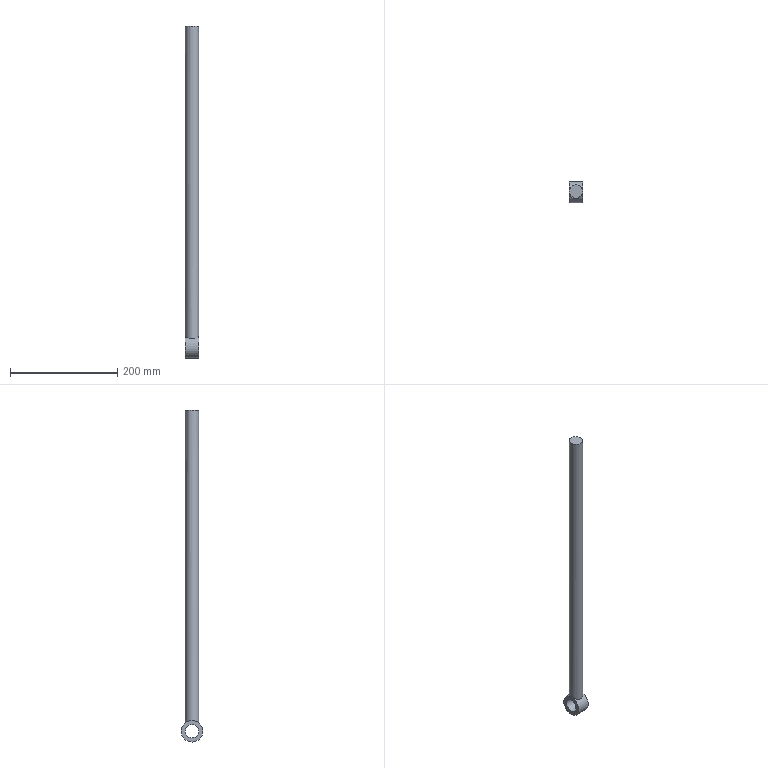Part | NX | features DATUM_CSYS 3, EXTRUDE 2, SKETCH 2, HOLE PACKAGE 1, SIMPLE HOLE 1 | 1 solid | 6 faces | box 25 x 40 x 620 mm | volume 304356 mm3 | cylinder 3 | plane 3 | commonest cylinder face diameters 25 x2 40 x1
STEP:
#1=CARTESIAN_POINT('',(12.5,0.,600.));
#2=VERTEX_POINT('',#1);
#3=CARTESIAN_POINT('',(0.,0.,600.));
#4=DIRECTION('',(0.,0.,1.));
#5=DIRECTION('',(1.,0.,0.));
#6=AXIS2_PLACEMENT_3D('',#3,#4,#5);
#7=CIRCLE('',#6,12.5);
#8=EDGE_CURVE('',#2,#2,#7,.T.);
#9=ORIENTED_EDGE('',*,*,#8,.F.);
#10=EDGE_LOOP('',(#9));
#11=FACE_BOUND('',#10,.T.);
#12=CARTESIAN_POINT('',(12.5,0.,20.));
#13=VERTEX_POINT('',#12);
#14=CARTESIAN_POINT('',(-12.5,0.,20.));
#15=VERTEX_POINT('',#14);
#16=CARTESIAN_POINT('',(12.5,0.,20.));
#17=CARTESIAN_POINT('',(12.5,-1.702,20.));
#18=CARTESIAN_POINT('',(11.797,-5.034,19.549));
#19=CARTESIAN_POINT('',(9.02,-9.08,17.957));
#20=CARTESIAN_POINT('',(5.048,-11.785,16.213));
#21=CARTESIAN_POINT('',(0.003287,-12.855,15.314));
#22=CARTESIAN_POINT('',(-5.025,-11.796,16.206));
#23=CARTESIAN_POINT('',(-9.03,-9.074,17.961));
#24=CARTESIAN_POINT('',(-11.795,-5.031,19.549));
#25=CARTESIAN_POINT('',(-12.5,-1.706,20.));
#26=CARTESIAN_POINT('',(-12.5,0.,20.));
#27=B_SPLINE_CURVE_WITH_KNOTS('',3,(#16,#17,#18,#19,#20,#21,#22,#23,#24,#25,#26),.UNSPECIFIED.,.F.,.F.,(4,1,1,1,1,1,1,1,4),(0.,0.005026,0.01005,0.01508,0.0201,0.02513,0.03016,0.03518,0.04021),.UNSPECIFIED.);
#28=EDGE_CURVE('',#13,#15,#27,.T.);
#29=ORIENTED_EDGE('',*,*,#28,.F.);
#30=CARTESIAN_POINT('',(-12.5,0.,20.));
#31=CARTESIAN_POINT('',(-12.5,1.702,20.));
#32=CARTESIAN_POINT('',(-11.797,5.034,19.549));
#33=CARTESIAN_POINT('',(-9.02,9.08,17.957));
#34=CARTESIAN_POINT('',(-5.048,11.785,16.213));
#35=CARTESIAN_POINT('',(-0.003287,12.855,15.314));
#36=CARTESIAN_POINT('',(5.025,11.796,16.206));
#37=CARTESIAN_POINT('',(9.03,9.074,17.961));
#38=CARTESIAN_POINT('',(11.795,5.031,19.549));
#39=CARTESIAN_POINT('',(12.5,1.706,20.));
#40=CARTESIAN_POINT('',(12.5,0.,20.));
#41=B_SPLINE_CURVE_WITH_KNOTS('',3,(#30,#31,#32,#33,#34,#35,#36,#37,#38,#39,#40),.UNSPECIFIED.,.F.,.F.,(4,1,1,1,1,1,1,1,4),(0.,0.005026,0.01005,0.01508,0.0201,0.02513,0.03016,0.03518,0.04021),.UNSPECIFIED.);
#42=EDGE_CURVE('',#15,#13,#41,.T.);
#43=ORIENTED_EDGE('',*,*,#42,.F.);
#44=EDGE_LOOP('',(#29,#43));
#45=FACE_BOUND('',#44,.T.);
#46=CARTESIAN_POINT('',(0.,0.,600.));
#47=DIRECTION('',(0.,0.,-1.));
#48=DIRECTION('',(-1.,0.,0.));
#49=AXIS2_PLACEMENT_3D('',#46,#47,#48);
#50=CYLINDRICAL_SURFACE('',#49,12.5);
#51=ADVANCED_FACE('',(#11,#45),#50,.T.);
#52=ORIENTED_EDGE('',*,*,#8,.T.);
#53=EDGE_LOOP('',(#52));
#54=FACE_BOUND('',#53,.T.);
#55=CARTESIAN_POINT('',(0.,0.,600.));
#56=DIRECTION('',(0.,0.,1.));
#57=DIRECTION('',(1.,0.,0.));
#58=AXIS2_PLACEMENT_3D('',#55,#56,#57);
#59=PLANE('',#58);
#60=ADVANCED_FACE('',(#54),#59,.T.);
#61=CARTESIAN_POINT('',(12.5,0.,0.));
#62=DIRECTION('',(1.,0.,0.));
#63=DIRECTION('',(0.,1.,0.));
#64=AXIS2_PLACEMENT_3D('',#61,#62,#63);
#65=CIRCLE('',#64,20.);
#66=EDGE_CURVE('',#13,#13,#65,.T.);
#67=ORIENTED_EDGE('',*,*,#66,.F.);
#68=ORIENTED_EDGE('',*,*,#28,.T.);
#69=CARTESIAN_POINT('',(-12.5,0.,0.));
#70=DIRECTION('',(1.,0.,0.));
#71=DIRECTION('',(0.,1.,0.));
#72=AXIS2_PLACEMENT_3D('',#69,#70,#71);
#73=CIRCLE('',#72,20.);
#74=EDGE_CURVE('',#15,#15,#73,.T.);
#75=ORIENTED_EDGE('',*,*,#74,.T.);
#76=ORIENTED_EDGE('',*,*,#42,.T.);
#77=EDGE_LOOP('',(#67,#68,#75,#76));
#78=FACE_BOUND('',#77,.T.);
#79=CARTESIAN_POINT('',(12.5,0.,0.));
#80=DIRECTION('',(-1.,0.,0.));
#81=DIRECTION('',(0.,0.,1.));
#82=AXIS2_PLACEMENT_3D('',#79,#80,#81);
#83=CYLINDRICAL_SURFACE('',#82,20.);
#84=ADVANCED_FACE('',(#78),#83,.T.);
#85=CARTESIAN_POINT('',(12.5,0.,-12.5));
#86=VERTEX_POINT('',#85);
#87=CARTESIAN_POINT('',(12.5,0.,0.));
#88=DIRECTION('',(1.,0.,0.));
#89=DIRECTION('',(0.,0.,-1.));
#90=AXIS2_PLACEMENT_3D('',#87,#88,#89);
#91=CIRCLE('',#90,12.5);
#92=EDGE_CURVE('',#86,#86,#91,.T.);
#93=ORIENTED_EDGE('',*,*,#92,.F.);
#94=EDGE_LOOP('',(#93));
#95=FACE_BOUND('',#94,.T.);
#96=ORIENTED_EDGE('',*,*,#66,.T.);
#97=EDGE_LOOP('',(#96));
#98=FACE_BOUND('',#97,.T.);
#99=CARTESIAN_POINT('',(12.5,0.,0.));
#100=DIRECTION('',(1.,0.,0.));
#101=DIRECTION('',(0.,0.,-1.));
#102=AXIS2_PLACEMENT_3D('',#99,#100,#101);
#103=PLANE('',#102);
#104=ADVANCED_FACE('',(#95,#98),#103,.T.);
#105=CARTESIAN_POINT('',(-12.5,0.,-12.5));
#106=VERTEX_POINT('',#105);
#107=CARTESIAN_POINT('',(-12.5,0.,0.));
#108=DIRECTION('',(1.,0.,0.));
#109=DIRECTION('',(0.,0.,-1.));
#110=AXIS2_PLACEMENT_3D('',#107,#108,#109);
#111=CIRCLE('',#110,12.5);
#112=EDGE_CURVE('',#106,#106,#111,.T.);
#113=ORIENTED_EDGE('',*,*,#112,.T.);
#114=EDGE_LOOP('',(#113));
#115=FACE_BOUND('',#114,.T.);
#116=ORIENTED_EDGE('',*,*,#74,.F.);
#117=EDGE_LOOP('',(#116));
#118=FACE_BOUND('',#117,.T.);
#119=CARTESIAN_POINT('',(-12.5,0.,0.));
#120=DIRECTION('',(1.,0.,0.));
#121=DIRECTION('',(0.,0.,-1.));
#122=AXIS2_PLACEMENT_3D('',#119,#120,#121);
#123=PLANE('',#122);
#124=ADVANCED_FACE('',(#115,#118),#123,.F.);
#125=ORIENTED_EDGE('',*,*,#92,.T.);
#126=EDGE_LOOP('',(#125));
#127=FACE_BOUND('',#126,.T.);
#128=ORIENTED_EDGE('',*,*,#112,.F.);
#129=EDGE_LOOP('',(#128));
#130=FACE_BOUND('',#129,.T.);
#131=CARTESIAN_POINT('',(-12.5,0.,0.));
#132=DIRECTION('',(1.,0.,0.));
#133=DIRECTION('',(0.,0.,-1.));
#134=AXIS2_PLACEMENT_3D('',#131,#132,#133);
#135=CYLINDRICAL_SURFACE('',#134,12.5);
#136=ADVANCED_FACE('',(#127,#130),#135,.F.);
#137=CLOSED_SHELL('',(#51,#60,#84,#104,#124,#136));
#138=MANIFOLD_SOLID_BREP('',#137);
#139=(LENGTH_UNIT()NAMED_UNIT(*)SI_UNIT(.MILLI.,.METRE.));
#140=UNCERTAINTY_MEASURE_WITH_UNIT(LENGTH_MEASURE(0.0508),#139,'','');
#141=(NAMED_UNIT(*)PLANE_ANGLE_UNIT()SI_UNIT($,.RADIAN.));
#142=(NAMED_UNIT(*)SI_UNIT($,.STERADIAN.)SOLID_ANGLE_UNIT());
#143=(GEOMETRIC_REPRESENTATION_CONTEXT(3)GLOBAL_UNCERTAINTY_ASSIGNED_CONTEXT((#140))GLOBAL_UNIT_ASSIGNED_CONTEXT((#139,#141,#142))REPRESENTATION_CONTEXT('',''));
#144=ADVANCED_BREP_SHAPE_REPRESENTATION('',(#138),#143);